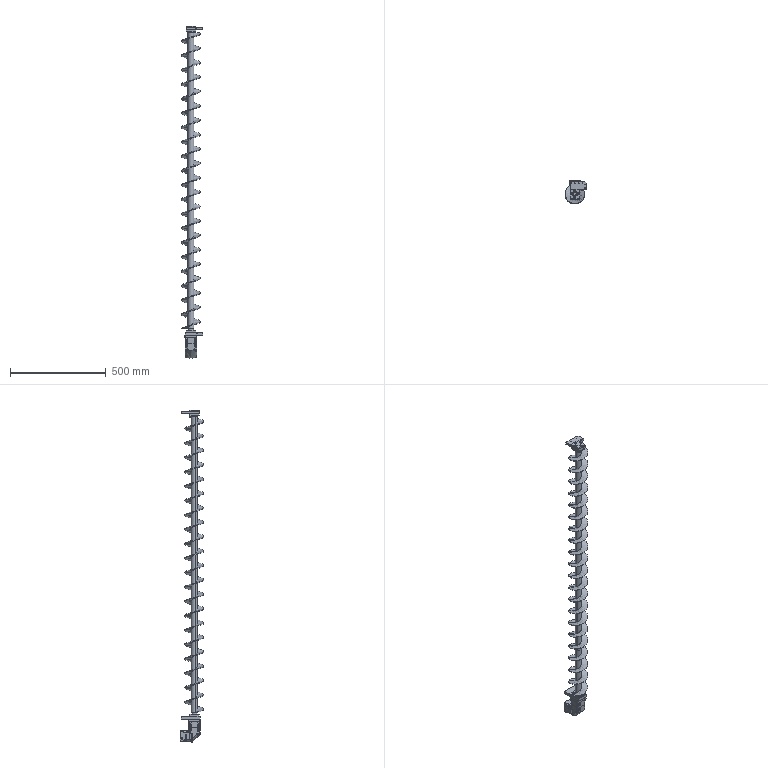Part | SolidWorks | features ReferencePattern 14, InContextFeatHolder 6, LocalLPattern 2 | 22 solids | 870 faces | box 112 x 125 x 1730 mm | volume 1536921 mm3 | cylinder 389 | plane 293 | cone 111 | spline 53 | torus 24 | commonest cylinder face diameters 4.2 x58 10 x36 69 x26 5.8 x24 3.3 x18 5.5 x16